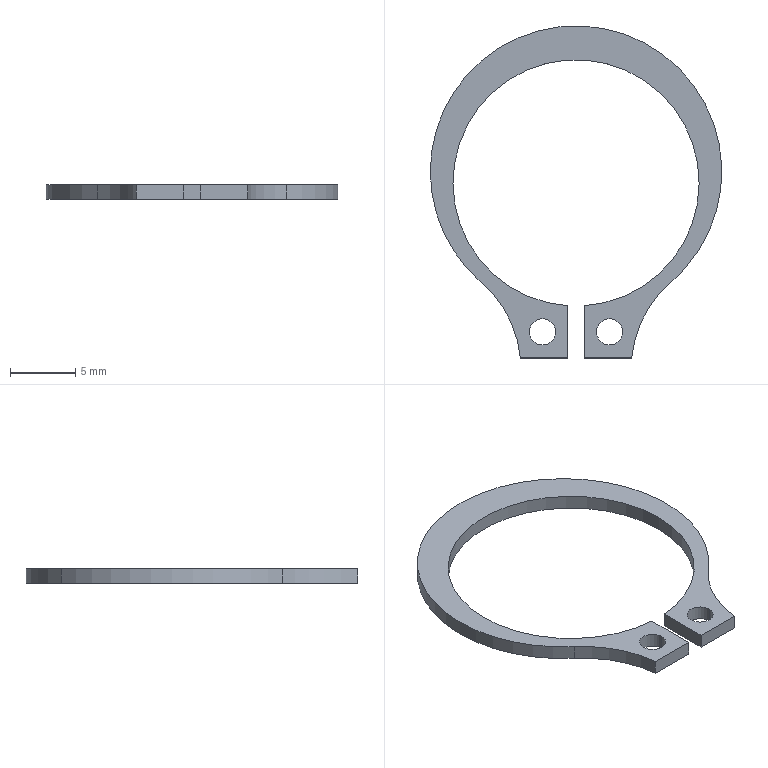Part | SolidWorks | features BaseBody 1 | 1 solid | 15 faces | box 22.317 x 25.426 x 1.1 mm | volume 148.534 mm3 | cylinder 9 | plane 6 | commonest cylinder face diameters 2 x4 17.382 x2 22.317 x2 18.85 x1
STEP:
#1=CARTESIAN_POINT('',(-1.567,-11.401,-1.1));
#2=VERTEX_POINT('',#1);
#3=CARTESIAN_POINT('',(-3.567,-11.401,-1.1));
#4=VERTEX_POINT('',#3);
#5=CARTESIAN_POINT('',(-2.567,-11.401,-1.1));
#6=DIRECTION('',(0.,0.,1.));
#7=DIRECTION('',(-1.,0.,0.));
#8=AXIS2_PLACEMENT_3D('',#5,#6,#7);
#9=CIRCLE('',#8,1.);
#10=EDGE_CURVE('',#2,#4,#9,.T.);
#11=ORIENTED_EDGE('',*,*,#10,.F.);
#12=CARTESIAN_POINT('',(-1.567,-11.401,0.));
#13=VERTEX_POINT('',#12);
#14=CARTESIAN_POINT('',(-1.567,-11.401,0.));
#15=DIRECTION('',(0.,0.,1.));
#16=VECTOR('',#15,1000.);
#17=LINE('',#14,#16);
#18=EDGE_CURVE('',#2,#13,#17,.T.);
#19=ORIENTED_EDGE('',*,*,#18,.T.);
#20=CARTESIAN_POINT('',(-3.567,-11.401,0.));
#21=VERTEX_POINT('',#20);
#22=CARTESIAN_POINT('',(-2.567,-11.401,0.));
#23=DIRECTION('',(0.,0.,-1.));
#24=DIRECTION('',(-1.,0.,0.));
#25=AXIS2_PLACEMENT_3D('',#22,#23,#24);
#26=CIRCLE('',#25,1.);
#27=EDGE_CURVE('',#21,#13,#26,.T.);
#28=ORIENTED_EDGE('',*,*,#27,.F.);
#29=CARTESIAN_POINT('',(-3.567,-11.401,0.));
#30=DIRECTION('',(0.,0.,1.));
#31=VECTOR('',#30,1000.);
#32=LINE('',#29,#31);
#33=EDGE_CURVE('',#4,#21,#32,.T.);
#34=ORIENTED_EDGE('',*,*,#33,.F.);
#35=EDGE_LOOP('',(#11,#19,#28,#34));
#36=FACE_OUTER_BOUND('',#35,.T.);
#37=CARTESIAN_POINT('',(-2.567,-11.401,0.));
#38=DIRECTION('',(0.,0.,1.));
#39=DIRECTION('',(-1.,0.,0.));
#40=AXIS2_PLACEMENT_3D('',#37,#38,#39);
#41=CYLINDRICAL_SURFACE('',#40,1.);
#42=ADVANCED_FACE('',(#36),#41,.F.);
#43=CARTESIAN_POINT('',(3.567,-11.401,-1.1));
#44=VERTEX_POINT('',#43);
#45=CARTESIAN_POINT('',(1.567,-11.401,-1.1));
#46=VERTEX_POINT('',#45);
#47=CARTESIAN_POINT('',(2.567,-11.401,-1.1));
#48=DIRECTION('',(0.,0.,1.));
#49=DIRECTION('',(-1.,0.,0.));
#50=AXIS2_PLACEMENT_3D('',#47,#48,#49);
#51=CIRCLE('',#50,1.);
#52=EDGE_CURVE('',#44,#46,#51,.T.);
#53=ORIENTED_EDGE('',*,*,#52,.F.);
#54=CARTESIAN_POINT('',(3.567,-11.401,0.));
#55=VERTEX_POINT('',#54);
#56=CARTESIAN_POINT('',(3.567,-11.401,0.));
#57=DIRECTION('',(0.,0.,1.));
#58=VECTOR('',#57,1000.);
#59=LINE('',#56,#58);
#60=EDGE_CURVE('',#44,#55,#59,.T.);
#61=ORIENTED_EDGE('',*,*,#60,.T.);
#62=CARTESIAN_POINT('',(1.567,-11.401,0.));
#63=VERTEX_POINT('',#62);
#64=CARTESIAN_POINT('',(2.567,-11.401,0.));
#65=DIRECTION('',(0.,0.,-1.));
#66=DIRECTION('',(-1.,0.,0.));
#67=AXIS2_PLACEMENT_3D('',#64,#65,#66);
#68=CIRCLE('',#67,1.);
#69=EDGE_CURVE('',#63,#55,#68,.T.);
#70=ORIENTED_EDGE('',*,*,#69,.F.);
#71=CARTESIAN_POINT('',(1.567,-11.401,0.));
#72=DIRECTION('',(0.,0.,1.));
#73=VECTOR('',#72,1000.);
#74=LINE('',#71,#73);
#75=EDGE_CURVE('',#46,#63,#74,.T.);
#76=ORIENTED_EDGE('',*,*,#75,.F.);
#77=EDGE_LOOP('',(#53,#61,#70,#76));
#78=FACE_OUTER_BOUND('',#77,.T.);
#79=CARTESIAN_POINT('',(2.567,-11.401,0.));
#80=DIRECTION('',(0.,0.,1.));
#81=DIRECTION('',(-1.,0.,0.));
#82=AXIS2_PLACEMENT_3D('',#79,#80,#81);
#83=CYLINDRICAL_SURFACE('',#82,1.);
#84=ADVANCED_FACE('',(#78),#83,.F.);
#85=CARTESIAN_POINT('',(7.263,-7.604,-1.1));
#86=VERTEX_POINT('',#85);
#87=CARTESIAN_POINT('',(-7.263,9.337,-1.1));
#88=VERTEX_POINT('',#87);
#89=CARTESIAN_POINT('',(0.,0.8667,-1.1));
#90=DIRECTION('',(0.,0.,1.));
#91=DIRECTION('',(-0.6509,0.7591,0.));
#92=AXIS2_PLACEMENT_3D('',#89,#90,#91);
#93=CIRCLE('',#92,11.158);
#94=EDGE_CURVE('',#86,#88,#93,.T.);
#95=ORIENTED_EDGE('',*,*,#94,.T.);
#96=CARTESIAN_POINT('',(-7.263,9.337,0.));
#97=VERTEX_POINT('',#96);
#98=CARTESIAN_POINT('',(-7.263,9.337,0.));
#99=DIRECTION('',(0.,0.,1.));
#100=VECTOR('',#99,1000.);
#101=LINE('',#98,#100);
#102=EDGE_CURVE('',#88,#97,#101,.T.);
#103=ORIENTED_EDGE('',*,*,#102,.T.);
#104=CARTESIAN_POINT('',(7.263,-7.604,0.));
#105=VERTEX_POINT('',#104);
#106=CARTESIAN_POINT('',(0.,0.8667,0.));
#107=DIRECTION('',(0.,0.,-1.));
#108=DIRECTION('',(-0.6509,0.7591,0.));
#109=AXIS2_PLACEMENT_3D('',#106,#107,#108);
#110=CIRCLE('',#109,11.158);
#111=EDGE_CURVE('',#97,#105,#110,.T.);
#112=ORIENTED_EDGE('',*,*,#111,.T.);
#113=CARTESIAN_POINT('',(7.263,-7.604,0.));
#114=DIRECTION('',(0.,0.,-1.));
#115=VECTOR('',#114,1000.);
#116=LINE('',#113,#115);
#117=EDGE_CURVE('',#105,#86,#116,.T.);
#118=ORIENTED_EDGE('',*,*,#117,.T.);
#119=EDGE_LOOP('',(#95,#103,#112,#118));
#120=FACE_OUTER_BOUND('',#119,.T.);
#121=CARTESIAN_POINT('',(0.,0.8667,0.));
#122=DIRECTION('',(0.,0.,1.));
#123=DIRECTION('',(-0.6509,0.7591,0.));
#124=AXIS2_PLACEMENT_3D('',#121,#122,#123);
#125=CYLINDRICAL_SURFACE('',#124,11.158);
#126=ADVANCED_FACE('',(#120),#125,.T.);
#127=CARTESIAN_POINT('',(-0.6667,-13.401,-1.1));
#128=VERTEX_POINT('',#127);
#129=CARTESIAN_POINT('',(-0.6667,-9.401,-1.1));
#130=VERTEX_POINT('',#129);
#131=CARTESIAN_POINT('',(-0.6667,-9.401,-1.1));
#132=DIRECTION('',(0.,1.,0.));
#133=VECTOR('',#132,1000.);
#134=LINE('',#131,#133);
#135=EDGE_CURVE('',#128,#130,#134,.T.);
#136=ORIENTED_EDGE('',*,*,#135,.T.);
#137=CARTESIAN_POINT('',(-0.6667,-9.401,0.));
#138=VERTEX_POINT('',#137);
#139=CARTESIAN_POINT('',(-0.6667,-9.401,0.));
#140=DIRECTION('',(0.,0.,-1.));
#141=VECTOR('',#140,1000.);
#142=LINE('',#139,#141);
#143=EDGE_CURVE('',#138,#130,#142,.T.);
#144=ORIENTED_EDGE('',*,*,#143,.F.);
#145=CARTESIAN_POINT('',(-0.6667,-13.401,0.));
#146=VERTEX_POINT('',#145);
#147=CARTESIAN_POINT('',(-0.6667,-9.401,0.));
#148=DIRECTION('',(0.,-1.,0.));
#149=VECTOR('',#148,1000.);
#150=LINE('',#147,#149);
#151=EDGE_CURVE('',#138,#146,#150,.T.);
#152=ORIENTED_EDGE('',*,*,#151,.T.);
#153=CARTESIAN_POINT('',(-0.6667,-13.401,0.));
#154=DIRECTION('',(0.,0.,-1.));
#155=VECTOR('',#154,1000.);
#156=LINE('',#153,#155);
#157=EDGE_CURVE('',#146,#128,#156,.T.);
#158=ORIENTED_EDGE('',*,*,#157,.T.);
#159=EDGE_LOOP('',(#136,#144,#152,#158));
#160=FACE_OUTER_BOUND('',#159,.T.);
#161=CARTESIAN_POINT('',(-0.6667,-13.401,0.));
#162=DIRECTION('',(1.,0.,0.));
#163=DIRECTION('',(0.,1.,0.));
#164=AXIS2_PLACEMENT_3D('',#161,#162,#163);
#165=PLANE('',#164);
#166=ADVANCED_FACE('',(#160),#165,.T.);
#167=CARTESIAN_POINT('',(0.6667,-9.401,-1.1));
#168=VERTEX_POINT('',#167);
#169=CARTESIAN_POINT('',(0.,0.,-1.1));
#170=DIRECTION('',(0.,0.,-1.));
#171=DIRECTION('',(0.07073,-0.9975,0.));
#172=AXIS2_PLACEMENT_3D('',#169,#170,#171);
#173=CIRCLE('',#172,9.425);
#174=EDGE_CURVE('',#130,#168,#173,.T.);
#175=ORIENTED_EDGE('',*,*,#174,.T.);
#176=CARTESIAN_POINT('',(0.6667,-9.401,0.));
#177=VERTEX_POINT('',#176);
#178=CARTESIAN_POINT('',(0.6667,-9.401,0.));
#179=DIRECTION('',(0.,0.,-1.));
#180=VECTOR('',#179,1000.);
#181=LINE('',#178,#180);
#182=EDGE_CURVE('',#177,#168,#181,.T.);
#183=ORIENTED_EDGE('',*,*,#182,.F.);
#184=CARTESIAN_POINT('',(0.,0.,0.));
#185=DIRECTION('',(0.,0.,1.));
#186=DIRECTION('',(0.07073,-0.9975,0.));
#187=AXIS2_PLACEMENT_3D('',#184,#185,#186);
#188=CIRCLE('',#187,9.425);
#189=EDGE_CURVE('',#177,#138,#188,.T.);
#190=ORIENTED_EDGE('',*,*,#189,.T.);
#191=ORIENTED_EDGE('',*,*,#143,.T.);
#192=EDGE_LOOP('',(#175,#183,#190,#191));
#193=FACE_OUTER_BOUND('',#192,.T.);
#194=CARTESIAN_POINT('',(0.,0.,0.));
#195=DIRECTION('',(0.,0.,1.));
#196=DIRECTION('',(0.07073,-0.9975,0.));
#197=AXIS2_PLACEMENT_3D('',#194,#195,#196);
#198=CYLINDRICAL_SURFACE('',#197,9.425);
#199=ADVANCED_FACE('',(#193),#198,.F.);
#200=CARTESIAN_POINT('',(0.6667,-13.401,-1.1));
#201=VERTEX_POINT('',#200);
#202=CARTESIAN_POINT('',(0.6667,-13.401,-1.1));
#203=DIRECTION('',(0.,-1.,0.));
#204=VECTOR('',#203,1000.);
#205=LINE('',#202,#204);
#206=EDGE_CURVE('',#168,#201,#205,.T.);
#207=ORIENTED_EDGE('',*,*,#206,.T.);
#208=CARTESIAN_POINT('',(0.6667,-13.401,0.));
#209=VERTEX_POINT('',#208);
#210=CARTESIAN_POINT('',(0.6667,-13.401,0.));
#211=DIRECTION('',(0.,0.,-1.));
#212=VECTOR('',#211,1000.);
#213=LINE('',#210,#212);
#214=EDGE_CURVE('',#209,#201,#213,.T.);
#215=ORIENTED_EDGE('',*,*,#214,.F.);
#216=CARTESIAN_POINT('',(0.6667,-13.401,0.));
#217=DIRECTION('',(0.,1.,0.));
#218=VECTOR('',#217,1000.);
#219=LINE('',#216,#218);
#220=EDGE_CURVE('',#209,#177,#219,.T.);
#221=ORIENTED_EDGE('',*,*,#220,.T.);
#222=ORIENTED_EDGE('',*,*,#182,.T.);
#223=EDGE_LOOP('',(#207,#215,#221,#222));
#224=FACE_OUTER_BOUND('',#223,.T.);
#225=CARTESIAN_POINT('',(0.6667,-9.401,0.));
#226=DIRECTION('',(-1.,0.,0.));
#227=DIRECTION('',(0.,0.,1.));
#228=AXIS2_PLACEMENT_3D('',#225,#226,#227);
#229=PLANE('',#228);
#230=ADVANCED_FACE('',(#224),#229,.T.);
#231=CARTESIAN_POINT('',(4.267,-13.401,-1.1));
#232=VERTEX_POINT('',#231);
#233=CARTESIAN_POINT('',(4.267,-13.401,-1.1));
#234=DIRECTION('',(1.,0.,0.));
#235=VECTOR('',#234,1000.);
#236=LINE('',#233,#235);
#237=EDGE_CURVE('',#201,#232,#236,.T.);
#238=ORIENTED_EDGE('',*,*,#237,.T.);
#239=CARTESIAN_POINT('',(4.267,-13.401,0.));
#240=VERTEX_POINT('',#239);
#241=CARTESIAN_POINT('',(4.267,-13.401,0.));
#242=DIRECTION('',(0.,0.,-1.));
#243=VECTOR('',#242,1000.);
#244=LINE('',#241,#243);
#245=EDGE_CURVE('',#240,#232,#244,.T.);
#246=ORIENTED_EDGE('',*,*,#245,.F.);
#247=CARTESIAN_POINT('',(4.267,-13.401,0.));
#248=DIRECTION('',(-1.,0.,0.));
#249=VECTOR('',#248,1000.);
#250=LINE('',#247,#249);
#251=EDGE_CURVE('',#240,#209,#250,.T.);
#252=ORIENTED_EDGE('',*,*,#251,.T.);
#253=ORIENTED_EDGE('',*,*,#214,.T.);
#254=EDGE_LOOP('',(#238,#246,#252,#253));
#255=FACE_OUTER_BOUND('',#254,.T.);
#256=CARTESIAN_POINT('',(0.6667,-13.401,0.));
#257=DIRECTION('',(0.,-1.,0.));
#258=DIRECTION('',(0.,0.,-1.));
#259=AXIS2_PLACEMENT_3D('',#256,#257,#258);
#260=PLANE('',#259);
#261=ADVANCED_FACE('',(#255),#260,.T.);
#262=CARTESIAN_POINT('',(12.921,-14.201,-1.1));
#263=DIRECTION('',(0.,0.,-1.));
#264=DIRECTION('',(-0.6509,0.7591,0.));
#265=AXIS2_PLACEMENT_3D('',#262,#263,#264);
#266=CIRCLE('',#265,8.691);
#267=EDGE_CURVE('',#232,#86,#266,.T.);
#268=ORIENTED_EDGE('',*,*,#267,.T.);
#269=ORIENTED_EDGE('',*,*,#117,.F.);
#270=CARTESIAN_POINT('',(12.921,-14.201,0.));
#271=DIRECTION('',(0.,0.,1.));
#272=DIRECTION('',(-0.6509,0.7591,0.));
#273=AXIS2_PLACEMENT_3D('',#270,#271,#272);
#274=CIRCLE('',#273,8.691);
#275=EDGE_CURVE('',#105,#240,#274,.T.);
#276=ORIENTED_EDGE('',*,*,#275,.T.);
#277=ORIENTED_EDGE('',*,*,#245,.T.);
#278=EDGE_LOOP('',(#268,#269,#276,#277));
#279=FACE_OUTER_BOUND('',#278,.T.);
#280=CARTESIAN_POINT('',(12.921,-14.201,0.));
#281=DIRECTION('',(0.,0.,1.));
#282=DIRECTION('',(-0.6509,0.7591,0.));
#283=AXIS2_PLACEMENT_3D('',#280,#281,#282);
#284=CYLINDRICAL_SURFACE('',#283,8.691);
#285=ADVANCED_FACE('',(#279),#284,.F.);
#286=CARTESIAN_POINT('',(-7.263,-7.604,-1.1));
#287=VERTEX_POINT('',#286);
#288=CARTESIAN_POINT('',(-4.267,-13.401,-1.1));
#289=VERTEX_POINT('',#288);
#290=CARTESIAN_POINT('',(-12.921,-14.201,-1.1));
#291=DIRECTION('',(0.,0.,-1.));
#292=DIRECTION('',(0.9958,0.09205,0.));
#293=AXIS2_PLACEMENT_3D('',#290,#291,#292);
#294=CIRCLE('',#293,8.691);
#295=EDGE_CURVE('',#287,#289,#294,.T.);
#296=ORIENTED_EDGE('',*,*,#295,.T.);
#297=CARTESIAN_POINT('',(-4.267,-13.401,0.));
#298=VERTEX_POINT('',#297);
#299=CARTESIAN_POINT('',(-4.267,-13.401,0.));
#300=DIRECTION('',(0.,0.,-1.));
#301=VECTOR('',#300,1000.);
#302=LINE('',#299,#301);
#303=EDGE_CURVE('',#298,#289,#302,.T.);
#304=ORIENTED_EDGE('',*,*,#303,.F.);
#305=CARTESIAN_POINT('',(-7.263,-7.604,0.));
#306=VERTEX_POINT('',#305);
#307=CARTESIAN_POINT('',(-12.921,-14.201,0.));
#308=DIRECTION('',(0.,0.,1.));
#309=DIRECTION('',(0.9958,0.09205,0.));
#310=AXIS2_PLACEMENT_3D('',#307,#308,#309);
#311=CIRCLE('',#310,8.691);
#312=EDGE_CURVE('',#298,#306,#311,.T.);
#313=ORIENTED_EDGE('',*,*,#312,.T.);
#314=CARTESIAN_POINT('',(-7.263,-7.604,0.));
#315=DIRECTION('',(0.,0.,-1.));
#316=VECTOR('',#315,1000.);
#317=LINE('',#314,#316);
#318=EDGE_CURVE('',#306,#287,#317,.T.);
#319=ORIENTED_EDGE('',*,*,#318,.T.);
#320=EDGE_LOOP('',(#296,#304,#313,#319));
#321=FACE_OUTER_BOUND('',#320,.T.);
#322=CARTESIAN_POINT('',(-12.921,-14.201,0.));
#323=DIRECTION('',(0.,0.,1.));
#324=DIRECTION('',(0.9958,0.09205,0.));
#325=AXIS2_PLACEMENT_3D('',#322,#323,#324);
#326=CYLINDRICAL_SURFACE('',#325,8.691);
#327=ADVANCED_FACE('',(#321),#326,.F.);
#328=CARTESIAN_POINT('',(-0.6667,-13.401,-1.1));
#329=DIRECTION('',(1.,0.,0.));
#330=VECTOR('',#329,1000.);
#331=LINE('',#328,#330);
#332=EDGE_CURVE('',#289,#128,#331,.T.);
#333=ORIENTED_EDGE('',*,*,#332,.T.);
#334=ORIENTED_EDGE('',*,*,#157,.F.);
#335=CARTESIAN_POINT('',(-0.6667,-13.401,0.));
#336=DIRECTION('',(-1.,0.,0.));
#337=VECTOR('',#336,1000.);
#338=LINE('',#335,#337);
#339=EDGE_CURVE('',#146,#298,#338,.T.);
#340=ORIENTED_EDGE('',*,*,#339,.T.);
#341=ORIENTED_EDGE('',*,*,#303,.T.);
#342=EDGE_LOOP('',(#333,#334,#340,#341));
#343=FACE_OUTER_BOUND('',#342,.T.);
#344=CARTESIAN_POINT('',(-4.267,-13.401,0.));
#345=DIRECTION('',(0.,-1.,0.));
#346=DIRECTION('',(-1.,0.,0.));
#347=AXIS2_PLACEMENT_3D('',#344,#345,#346);
#348=PLANE('',#347);
#349=ADVANCED_FACE('',(#343),#348,.T.);
#350=ORIENTED_EDGE('',*,*,#27,.T.);
#351=CARTESIAN_POINT('',(-2.567,-11.401,0.));
#352=DIRECTION('',(0.,0.,-1.));
#353=DIRECTION('',(-1.,0.,0.));
#354=AXIS2_PLACEMENT_3D('',#351,#352,#353);
#355=CIRCLE('',#354,1.);
#356=EDGE_CURVE('',#13,#21,#355,.T.);
#357=ORIENTED_EDGE('',*,*,#356,.T.);
#358=EDGE_LOOP('',(#350,#357));
#359=FACE_BOUND('',#358,.T.);
#360=ORIENTED_EDGE('',*,*,#69,.T.);
#361=CARTESIAN_POINT('',(2.567,-11.401,0.));
#362=DIRECTION('',(0.,0.,-1.));
#363=DIRECTION('',(-1.,0.,0.));
#364=AXIS2_PLACEMENT_3D('',#361,#362,#363);
#365=CIRCLE('',#364,1.);
#366=EDGE_CURVE('',#55,#63,#365,.T.);
#367=ORIENTED_EDGE('',*,*,#366,.T.);
#368=EDGE_LOOP('',(#360,#367));
#369=FACE_BOUND('',#368,.T.);
#370=ORIENTED_EDGE('',*,*,#339,.F.);
#371=ORIENTED_EDGE('',*,*,#151,.F.);
#372=ORIENTED_EDGE('',*,*,#189,.F.);
#373=ORIENTED_EDGE('',*,*,#220,.F.);
#374=ORIENTED_EDGE('',*,*,#251,.F.);
#375=ORIENTED_EDGE('',*,*,#275,.F.);
#376=ORIENTED_EDGE('',*,*,#111,.F.);
#377=CARTESIAN_POINT('',(0.,0.8667,0.));
#378=DIRECTION('',(0.,0.,-1.));
#379=DIRECTION('',(-0.6509,0.7591,0.));
#380=AXIS2_PLACEMENT_3D('',#377,#378,#379);
#381=CIRCLE('',#380,11.158);
#382=EDGE_CURVE('',#306,#97,#381,.T.);
#383=ORIENTED_EDGE('',*,*,#382,.F.);
#384=ORIENTED_EDGE('',*,*,#312,.F.);
#385=EDGE_LOOP('',(#370,#371,#372,#373,#374,#375,#376,#383,#384));
#386=FACE_OUTER_BOUND('',#385,.T.);
#387=CARTESIAN_POINT('',(0.,-1.525,0.));
#388=DIRECTION('',(0.,0.,1.));
#389=DIRECTION('',(1.,0.,0.));
#390=AXIS2_PLACEMENT_3D('',#387,#388,#389);
#391=PLANE('',#390);
#392=ADVANCED_FACE('',(#359,#369,#386),#391,.T.);
#393=CARTESIAN_POINT('',(-2.567,-11.401,-1.1));
#394=DIRECTION('',(0.,0.,1.));
#395=DIRECTION('',(-1.,0.,0.));
#396=AXIS2_PLACEMENT_3D('',#393,#394,#395);
#397=CIRCLE('',#396,1.);
#398=EDGE_CURVE('',#4,#2,#397,.T.);
#399=ORIENTED_EDGE('',*,*,#398,.T.);
#400=ORIENTED_EDGE('',*,*,#10,.T.);
#401=EDGE_LOOP('',(#399,#400));
#402=FACE_BOUND('',#401,.T.);
#403=CARTESIAN_POINT('',(2.567,-11.401,-1.1));
#404=DIRECTION('',(0.,0.,1.));
#405=DIRECTION('',(-1.,0.,0.));
#406=AXIS2_PLACEMENT_3D('',#403,#404,#405);
#407=CIRCLE('',#406,1.);
#408=EDGE_CURVE('',#46,#44,#407,.T.);
#409=ORIENTED_EDGE('',*,*,#408,.T.);
#410=ORIENTED_EDGE('',*,*,#52,.T.);
#411=EDGE_LOOP('',(#409,#410));
#412=FACE_BOUND('',#411,.T.);
#413=ORIENTED_EDGE('',*,*,#135,.F.);
#414=ORIENTED_EDGE('',*,*,#332,.F.);
#415=ORIENTED_EDGE('',*,*,#295,.F.);
#416=CARTESIAN_POINT('',(0.,0.8667,-1.1));
#417=DIRECTION('',(0.,0.,1.));
#418=DIRECTION('',(-0.6509,0.7591,0.));
#419=AXIS2_PLACEMENT_3D('',#416,#417,#418);
#420=CIRCLE('',#419,11.158);
#421=EDGE_CURVE('',#88,#287,#420,.T.);
#422=ORIENTED_EDGE('',*,*,#421,.F.);
#423=ORIENTED_EDGE('',*,*,#94,.F.);
#424=ORIENTED_EDGE('',*,*,#267,.F.);
#425=ORIENTED_EDGE('',*,*,#237,.F.);
#426=ORIENTED_EDGE('',*,*,#206,.F.);
#427=ORIENTED_EDGE('',*,*,#174,.F.);
#428=EDGE_LOOP('',(#413,#414,#415,#422,#423,#424,#425,#426,#427));
#429=FACE_OUTER_BOUND('',#428,.T.);
#430=CARTESIAN_POINT('',(0.,-1.525,-1.1));
#431=DIRECTION('',(0.,0.,1.));
#432=DIRECTION('',(1.,0.,0.));
#433=AXIS2_PLACEMENT_3D('',#430,#431,#432);
#434=PLANE('',#433);
#435=ADVANCED_FACE('',(#402,#412,#429),#434,.F.);
#436=ORIENTED_EDGE('',*,*,#102,.F.);
#437=ORIENTED_EDGE('',*,*,#421,.T.);
#438=ORIENTED_EDGE('',*,*,#318,.F.);
#439=ORIENTED_EDGE('',*,*,#382,.T.);
#440=EDGE_LOOP('',(#436,#437,#438,#439));
#441=FACE_OUTER_BOUND('',#440,.T.);
#442=CARTESIAN_POINT('',(0.,0.8667,0.));
#443=DIRECTION('',(0.,0.,1.));
#444=DIRECTION('',(-0.6509,0.7591,0.));
#445=AXIS2_PLACEMENT_3D('',#442,#443,#444);
#446=CYLINDRICAL_SURFACE('',#445,11.158);
#447=ADVANCED_FACE('',(#441),#446,.T.);
#448=ORIENTED_EDGE('',*,*,#60,.F.);
#449=ORIENTED_EDGE('',*,*,#408,.F.);
#450=ORIENTED_EDGE('',*,*,#75,.T.);
#451=ORIENTED_EDGE('',*,*,#366,.F.);
#452=EDGE_LOOP('',(#448,#449,#450,#451));
#453=FACE_OUTER_BOUND('',#452,.T.);
#454=CARTESIAN_POINT('',(2.567,-11.401,0.));
#455=DIRECTION('',(0.,0.,1.));
#456=DIRECTION('',(-1.,0.,0.));
#457=AXIS2_PLACEMENT_3D('',#454,#455,#456);
#458=CYLINDRICAL_SURFACE('',#457,1.);
#459=ADVANCED_FACE('',(#453),#458,.F.);
#460=ORIENTED_EDGE('',*,*,#18,.F.);
#461=ORIENTED_EDGE('',*,*,#398,.F.);
#462=ORIENTED_EDGE('',*,*,#33,.T.);
#463=ORIENTED_EDGE('',*,*,#356,.F.);
#464=EDGE_LOOP('',(#460,#461,#462,#463));
#465=FACE_OUTER_BOUND('',#464,.T.);
#466=CARTESIAN_POINT('',(-2.567,-11.401,0.));
#467=DIRECTION('',(0.,0.,1.));
#468=DIRECTION('',(-1.,0.,0.));
#469=AXIS2_PLACEMENT_3D('',#466,#467,#468);
#470=CYLINDRICAL_SURFACE('',#469,1.);
#471=ADVANCED_FACE('',(#465),#470,.F.);
#472=CLOSED_SHELL('',(#42,#84,#126,#166,#199,#230,#261,#285,#327,#349,#392,#435,#447,#459,#471));
#473=MANIFOLD_SOLID_BREP('',#472);
#474=CARTESIAN_POINT('',(0.,0.,0.));
#475=DIRECTION('',(0.,0.,1.));
#476=DIRECTION('',(1.,0.,0.));
#477=AXIS2_PLACEMENT_3D('',#474,#475,#476);
#478=(LENGTH_UNIT()NAMED_UNIT(*)SI_UNIT(.MILLI.,.METRE.));
#479=UNCERTAINTY_MEASURE_WITH_UNIT(LENGTH_MEASURE(0.00001),#478,'','');
#480=(NAMED_UNIT(*)PLANE_ANGLE_UNIT()SI_UNIT($,.RADIAN.));
#481=(NAMED_UNIT(*)SI_UNIT($,.STERADIAN.)SOLID_ANGLE_UNIT());
#482=(GEOMETRIC_REPRESENTATION_CONTEXT(3)GLOBAL_UNCERTAINTY_ASSIGNED_CONTEXT((#479))GLOBAL_UNIT_ASSIGNED_CONTEXT((#478,#480,#481))REPRESENTATION_CONTEXT('',''));
#483=ADVANCED_BREP_SHAPE_REPRESENTATION('',(#473,#477),#482);